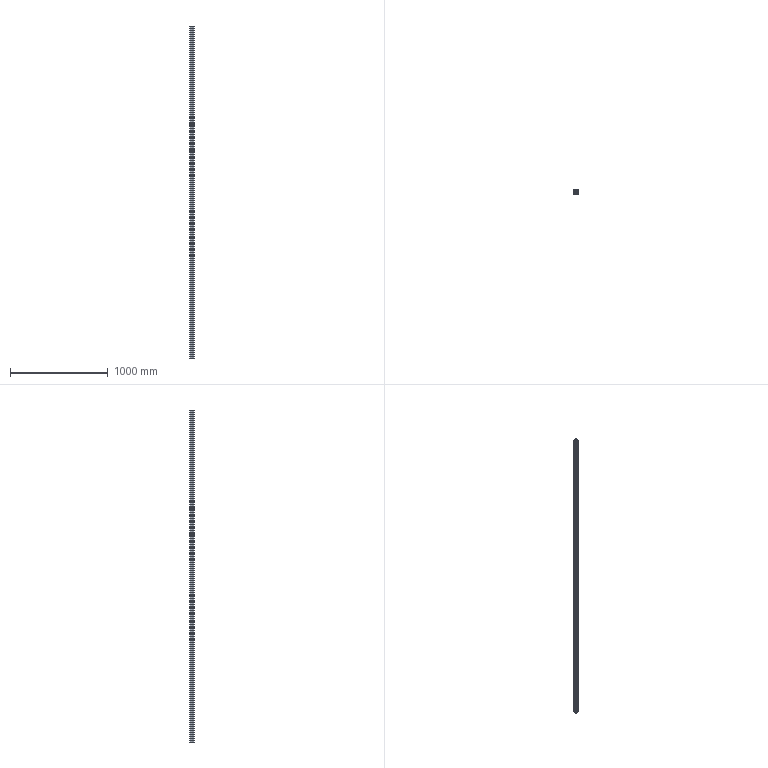Part | STEP file | BCC3 H13_5 | 1 solid | 107 faces | box 45 x 45 x 3395 mm | volume 4368342 mm3 | cylinder 57 | plane 50 | commonest cylinder face diameters 1 x32 2 x8 4 x8 23.17 x5 7 x4